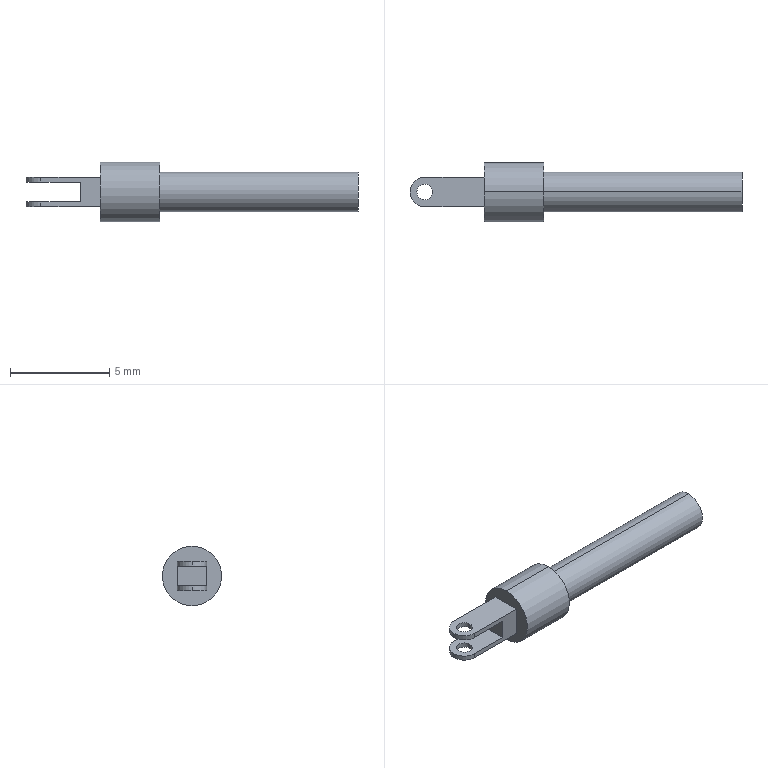Part | SolidWorks | features ICE 3, Revolution 1 | 1 solid | 25 faces | box 16.75 x 3 x 3 mm | volume 51.85 mm3 | cylinder 14 | plane 11 | commonest cylinder face diameters 0.8 x4 1.5 x4 1 x2 2 x2 3 x2
STEP:
#1=CARTESIAN_POINT('',(7.,0.,0.5));
#2=VERTEX_POINT('',#1);
#3=CARTESIAN_POINT('',(7.,0.,-0.5));
#4=VERTEX_POINT('',#3);
#5=CARTESIAN_POINT('',(7.,0.,0.));
#6=DIRECTION('',(1.,0.,0.));
#7=DIRECTION('',(0.,0.,-1.));
#8=AXIS2_PLACEMENT_3D('',#5,#6,#7);
#9=CIRCLE('',#8,0.5);
#10=EDGE_CURVE('',#2,#4,#9,.T.);
#11=ORIENTED_EDGE('',*,*,#10,.F.);
#12=CARTESIAN_POINT('',(13.,0.,0.5));
#13=VERTEX_POINT('',#12);
#14=CARTESIAN_POINT('',(7.,0.,0.5));
#15=DIRECTION('',(1.,0.,0.));
#16=VECTOR('',#15,1000.);
#17=LINE('',#14,#16);
#18=EDGE_CURVE('',#2,#13,#17,.T.);
#19=ORIENTED_EDGE('',*,*,#18,.T.);
#20=CARTESIAN_POINT('',(13.,0.,-0.5));
#21=VERTEX_POINT('',#20);
#22=CARTESIAN_POINT('',(13.,0.,0.));
#23=DIRECTION('',(1.,0.,0.));
#24=DIRECTION('',(0.,0.,-1.));
#25=AXIS2_PLACEMENT_3D('',#22,#23,#24);
#26=CIRCLE('',#25,0.5);
#27=EDGE_CURVE('',#13,#21,#26,.T.);
#28=ORIENTED_EDGE('',*,*,#27,.T.);
#29=CARTESIAN_POINT('',(7.,0.,-0.5));
#30=DIRECTION('',(1.,0.,0.));
#31=VECTOR('',#30,1000.);
#32=LINE('',#29,#31);
#33=EDGE_CURVE('',#4,#21,#32,.T.);
#34=ORIENTED_EDGE('',*,*,#33,.F.);
#35=EDGE_LOOP('',(#11,#19,#28,#34));
#36=FACE_OUTER_BOUND('',#35,.T.);
#37=CARTESIAN_POINT('',(7.,0.,0.));
#38=DIRECTION('',(1.,0.,0.));
#39=DIRECTION('',(0.,0.,-1.));
#40=AXIS2_PLACEMENT_3D('',#37,#38,#39);
#41=CYLINDRICAL_SURFACE('',#40,0.5);
#42=ADVANCED_FACE('',(#36),#41,.F.);
#43=CARTESIAN_POINT('',(-2.6,0.,-0.5));
#44=VERTEX_POINT('',#43);
#45=CARTESIAN_POINT('',(-3.4,0.,-0.5));
#46=VERTEX_POINT('',#45);
#47=CARTESIAN_POINT('',(-3.,0.,-0.5));
#48=DIRECTION('',(0.,0.,-1.));
#49=DIRECTION('',(-1.,0.,0.));
#50=AXIS2_PLACEMENT_3D('',#47,#48,#49);
#51=CIRCLE('',#50,0.4);
#52=EDGE_CURVE('',#44,#46,#51,.T.);
#53=ORIENTED_EDGE('',*,*,#52,.F.);
#54=CARTESIAN_POINT('',(-2.6,0.,-0.75));
#55=VERTEX_POINT('',#54);
#56=CARTESIAN_POINT('',(-2.6,0.,0.75));
#57=DIRECTION('',(0.,0.,-1.));
#58=VECTOR('',#57,1000.);
#59=LINE('',#56,#58);
#60=EDGE_CURVE('',#44,#55,#59,.T.);
#61=ORIENTED_EDGE('',*,*,#60,.T.);
#62=CARTESIAN_POINT('',(-3.4,0.,-0.75));
#63=VERTEX_POINT('',#62);
#64=CARTESIAN_POINT('',(-3.,0.,-0.75));
#65=DIRECTION('',(0.,0.,1.));
#66=DIRECTION('',(1.,0.,0.));
#67=AXIS2_PLACEMENT_3D('',#64,#65,#66);
#68=CIRCLE('',#67,0.4);
#69=EDGE_CURVE('',#63,#55,#68,.T.);
#70=ORIENTED_EDGE('',*,*,#69,.F.);
#71=CARTESIAN_POINT('',(-3.4,0.,0.75));
#72=DIRECTION('',(0.,0.,-1.));
#73=VECTOR('',#72,1000.);
#74=LINE('',#71,#73);
#75=EDGE_CURVE('',#46,#63,#74,.T.);
#76=ORIENTED_EDGE('',*,*,#75,.F.);
#77=EDGE_LOOP('',(#53,#61,#70,#76));
#78=FACE_OUTER_BOUND('',#77,.T.);
#79=CARTESIAN_POINT('',(-3.,0.,0.75));
#80=DIRECTION('',(0.,0.,-1.));
#81=DIRECTION('',(-1.,0.,0.));
#82=AXIS2_PLACEMENT_3D('',#79,#80,#81);
#83=CYLINDRICAL_SURFACE('',#82,0.4);
#84=ADVANCED_FACE('',(#78),#83,.F.);
#85=CARTESIAN_POINT('',(-3.75,0.,-0.5));
#86=VERTEX_POINT('',#85);
#87=CARTESIAN_POINT('',(-3.,-0.75,-0.5));
#88=VERTEX_POINT('',#87);
#89=CARTESIAN_POINT('',(-3.,0.,-0.5));
#90=DIRECTION('',(0.,0.,1.));
#91=DIRECTION('',(-1.,0.,0.));
#92=AXIS2_PLACEMENT_3D('',#89,#90,#91);
#93=CIRCLE('',#92,0.75);
#94=EDGE_CURVE('',#86,#88,#93,.T.);
#95=ORIENTED_EDGE('',*,*,#94,.F.);
#96=CARTESIAN_POINT('',(-3.75,0.,-0.75));
#97=VERTEX_POINT('',#96);
#98=CARTESIAN_POINT('',(-3.75,0.,0.75));
#99=DIRECTION('',(0.,0.,-1.));
#100=VECTOR('',#99,1000.);
#101=LINE('',#98,#100);
#102=EDGE_CURVE('',#86,#97,#101,.T.);
#103=ORIENTED_EDGE('',*,*,#102,.T.);
#104=CARTESIAN_POINT('',(-3.,-0.75,-0.75));
#105=VERTEX_POINT('',#104);
#106=CARTESIAN_POINT('',(-3.,0.,-0.75));
#107=DIRECTION('',(0.,0.,1.));
#108=DIRECTION('',(-1.,0.,0.));
#109=AXIS2_PLACEMENT_3D('',#106,#107,#108);
#110=CIRCLE('',#109,0.75);
#111=EDGE_CURVE('',#97,#105,#110,.T.);
#112=ORIENTED_EDGE('',*,*,#111,.T.);
#113=CARTESIAN_POINT('',(-3.,-0.75,0.75));
#114=DIRECTION('',(0.,0.,-1.));
#115=VECTOR('',#114,1000.);
#116=LINE('',#113,#115);
#117=EDGE_CURVE('',#88,#105,#116,.T.);
#118=ORIENTED_EDGE('',*,*,#117,.F.);
#119=EDGE_LOOP('',(#95,#103,#112,#118));
#120=FACE_OUTER_BOUND('',#119,.T.);
#121=CARTESIAN_POINT('',(-3.,0.,0.75));
#122=DIRECTION('',(0.,0.,-1.));
#123=DIRECTION('',(-1.,0.,0.));
#124=AXIS2_PLACEMENT_3D('',#121,#122,#123);
#125=CYLINDRICAL_SURFACE('',#124,0.75);
#126=ADVANCED_FACE('',(#120),#125,.T.);
#127=CARTESIAN_POINT('',(13.,0.,1.));
#128=VERTEX_POINT('',#127);
#129=CARTESIAN_POINT('',(13.,0.,-1.));
#130=VERTEX_POINT('',#129);
#131=CARTESIAN_POINT('',(13.,0.,0.));
#132=DIRECTION('',(-1.,0.,0.));
#133=DIRECTION('',(0.,0.,1.));
#134=AXIS2_PLACEMENT_3D('',#131,#132,#133);
#135=CIRCLE('',#134,1.);
#136=EDGE_CURVE('',#128,#130,#135,.T.);
#137=ORIENTED_EDGE('',*,*,#136,.T.);
#138=CARTESIAN_POINT('',(3.,0.,-1.));
#139=VERTEX_POINT('',#138);
#140=CARTESIAN_POINT('',(0.1244,0.,-1.));
#141=DIRECTION('',(-1.,0.,0.));
#142=VECTOR('',#141,1000.);
#143=LINE('',#140,#142);
#144=EDGE_CURVE('',#130,#139,#143,.T.);
#145=ORIENTED_EDGE('',*,*,#144,.T.);
#146=CARTESIAN_POINT('',(3.,0.,1.));
#147=VERTEX_POINT('',#146);
#148=CARTESIAN_POINT('',(3.,0.,0.));
#149=DIRECTION('',(-1.,0.,0.));
#150=DIRECTION('',(0.,0.,1.));
#151=AXIS2_PLACEMENT_3D('',#148,#149,#150);
#152=CIRCLE('',#151,1.);
#153=EDGE_CURVE('',#147,#139,#152,.T.);
#154=ORIENTED_EDGE('',*,*,#153,.F.);
#155=CARTESIAN_POINT('',(0.1244,0.,1.));
#156=DIRECTION('',(-1.,0.,0.));
#157=VECTOR('',#156,1000.);
#158=LINE('',#155,#157);
#159=EDGE_CURVE('',#128,#147,#158,.T.);
#160=ORIENTED_EDGE('',*,*,#159,.F.);
#161=EDGE_LOOP('',(#137,#145,#154,#160));
#162=FACE_OUTER_BOUND('',#161,.T.);
#163=CARTESIAN_POINT('',(0.1244,0.,0.));
#164=DIRECTION('',(-1.,0.,0.));
#165=DIRECTION('',(0.,0.,1.));
#166=AXIS2_PLACEMENT_3D('',#163,#164,#165);
#167=CYLINDRICAL_SURFACE('',#166,1.);
#168=ADVANCED_FACE('',(#162),#167,.T.);
#169=CARTESIAN_POINT('',(3.,0.,1.5));
#170=VERTEX_POINT('',#169);
#171=CARTESIAN_POINT('',(3.,0.,-1.5));
#172=VERTEX_POINT('',#171);
#173=CARTESIAN_POINT('',(3.,0.,0.));
#174=DIRECTION('',(-1.,0.,0.));
#175=DIRECTION('',(0.,0.,1.));
#176=AXIS2_PLACEMENT_3D('',#173,#174,#175);
#177=CIRCLE('',#176,1.5);
#178=EDGE_CURVE('',#170,#172,#177,.T.);
#179=ORIENTED_EDGE('',*,*,#178,.T.);
#180=CARTESIAN_POINT('',(0.,0.,-1.5));
#181=VERTEX_POINT('',#180);
#182=CARTESIAN_POINT('',(0.1244,0.,-1.5));
#183=DIRECTION('',(-1.,0.,0.));
#184=VECTOR('',#183,1000.);
#185=LINE('',#182,#184);
#186=EDGE_CURVE('',#172,#181,#185,.T.);
#187=ORIENTED_EDGE('',*,*,#186,.T.);
#188=CARTESIAN_POINT('',(0.,0.,1.5));
#189=VERTEX_POINT('',#188);
#190=CARTESIAN_POINT('',(0.,0.,0.));
#191=DIRECTION('',(-1.,0.,0.));
#192=DIRECTION('',(0.,0.,1.));
#193=AXIS2_PLACEMENT_3D('',#190,#191,#192);
#194=CIRCLE('',#193,1.5);
#195=EDGE_CURVE('',#189,#181,#194,.T.);
#196=ORIENTED_EDGE('',*,*,#195,.F.);
#197=CARTESIAN_POINT('',(0.1244,0.,1.5));
#198=DIRECTION('',(-1.,0.,0.));
#199=VECTOR('',#198,1000.);
#200=LINE('',#197,#199);
#201=EDGE_CURVE('',#170,#189,#200,.T.);
#202=ORIENTED_EDGE('',*,*,#201,.F.);
#203=EDGE_LOOP('',(#179,#187,#196,#202));
#204=FACE_OUTER_BOUND('',#203,.T.);
#205=CARTESIAN_POINT('',(0.1244,0.,0.));
#206=DIRECTION('',(-1.,0.,0.));
#207=DIRECTION('',(0.,0.,1.));
#208=AXIS2_PLACEMENT_3D('',#205,#206,#207);
#209=CYLINDRICAL_SURFACE('',#208,1.5);
#210=ADVANCED_FACE('',(#204),#209,.T.);
#211=CARTESIAN_POINT('',(-3.4,0.,0.75));
#212=VERTEX_POINT('',#211);
#213=CARTESIAN_POINT('',(-2.6,0.,0.75));
#214=VERTEX_POINT('',#213);
#215=CARTESIAN_POINT('',(-3.,0.,0.75));
#216=DIRECTION('',(0.,0.,1.));
#217=DIRECTION('',(1.,0.,0.));
#218=AXIS2_PLACEMENT_3D('',#215,#216,#217);
#219=CIRCLE('',#218,0.4);
#220=EDGE_CURVE('',#212,#214,#219,.T.);
#221=ORIENTED_EDGE('',*,*,#220,.T.);
#222=CARTESIAN_POINT('',(-2.6,0.,0.5));
#223=VERTEX_POINT('',#222);
#224=CARTESIAN_POINT('',(-2.6,0.,0.75));
#225=DIRECTION('',(0.,0.,-1.));
#226=VECTOR('',#225,1000.);
#227=LINE('',#224,#226);
#228=EDGE_CURVE('',#214,#223,#227,.T.);
#229=ORIENTED_EDGE('',*,*,#228,.T.);
#230=CARTESIAN_POINT('',(-3.4,0.,0.5));
#231=VERTEX_POINT('',#230);
#232=CARTESIAN_POINT('',(-3.,0.,0.5));
#233=DIRECTION('',(0.,0.,-1.));
#234=DIRECTION('',(-1.,0.,0.));
#235=AXIS2_PLACEMENT_3D('',#232,#233,#234);
#236=CIRCLE('',#235,0.4);
#237=EDGE_CURVE('',#223,#231,#236,.T.);
#238=ORIENTED_EDGE('',*,*,#237,.T.);
#239=CARTESIAN_POINT('',(-3.4,0.,0.75));
#240=DIRECTION('',(0.,0.,-1.));
#241=VECTOR('',#240,1000.);
#242=LINE('',#239,#241);
#243=EDGE_CURVE('',#212,#231,#242,.T.);
#244=ORIENTED_EDGE('',*,*,#243,.F.);
#245=EDGE_LOOP('',(#221,#229,#238,#244));
#246=FACE_OUTER_BOUND('',#245,.T.);
#247=CARTESIAN_POINT('',(-3.,0.,0.75));
#248=DIRECTION('',(0.,0.,-1.));
#249=DIRECTION('',(-1.,0.,0.));
#250=AXIS2_PLACEMENT_3D('',#247,#248,#249);
#251=CYLINDRICAL_SURFACE('',#250,0.4);
#252=ADVANCED_FACE('',(#246),#251,.F.);
#253=CARTESIAN_POINT('',(-3.75,0.,0.75));
#254=VERTEX_POINT('',#253);
#255=CARTESIAN_POINT('',(-3.,-0.75,0.75));
#256=VERTEX_POINT('',#255);
#257=CARTESIAN_POINT('',(-3.,0.,0.75));
#258=DIRECTION('',(0.,0.,1.));
#259=DIRECTION('',(-1.,0.,0.));
#260=AXIS2_PLACEMENT_3D('',#257,#258,#259);
#261=CIRCLE('',#260,0.75);
#262=EDGE_CURVE('',#254,#256,#261,.T.);
#263=ORIENTED_EDGE('',*,*,#262,.F.);
#264=CARTESIAN_POINT('',(-3.75,0.,0.5));
#265=VERTEX_POINT('',#264);
#266=CARTESIAN_POINT('',(-3.75,0.,0.75));
#267=DIRECTION('',(0.,0.,-1.));
#268=VECTOR('',#267,1000.);
#269=LINE('',#266,#268);
#270=EDGE_CURVE('',#254,#265,#269,.T.);
#271=ORIENTED_EDGE('',*,*,#270,.T.);
#272=CARTESIAN_POINT('',(-3.,-0.75,0.5));
#273=VERTEX_POINT('',#272);
#274=CARTESIAN_POINT('',(-3.,0.,0.5));
#275=DIRECTION('',(0.,0.,1.));
#276=DIRECTION('',(-1.,0.,0.));
#277=AXIS2_PLACEMENT_3D('',#274,#275,#276);
#278=CIRCLE('',#277,0.75);
#279=EDGE_CURVE('',#265,#273,#278,.T.);
#280=ORIENTED_EDGE('',*,*,#279,.T.);
#281=CARTESIAN_POINT('',(-3.,-0.75,0.75));
#282=DIRECTION('',(0.,0.,-1.));
#283=VECTOR('',#282,1000.);
#284=LINE('',#281,#283);
#285=EDGE_CURVE('',#256,#273,#284,.T.);
#286=ORIENTED_EDGE('',*,*,#285,.F.);
#287=EDGE_LOOP('',(#263,#271,#280,#286));
#288=FACE_OUTER_BOUND('',#287,.T.);
#289=CARTESIAN_POINT('',(-3.,0.,0.75));
#290=DIRECTION('',(0.,0.,-1.));
#291=DIRECTION('',(-1.,0.,0.));
#292=AXIS2_PLACEMENT_3D('',#289,#290,#291);
#293=CYLINDRICAL_SURFACE('',#292,0.75);
#294=ADVANCED_FACE('',(#288),#293,.T.);
#295=ORIENTED_EDGE('',*,*,#270,.F.);
#296=CARTESIAN_POINT('',(-3.,0.75,0.75));
#297=VERTEX_POINT('',#296);
#298=CARTESIAN_POINT('',(-3.,0.,0.75));
#299=DIRECTION('',(0.,0.,1.));
#300=DIRECTION('',(-1.,0.,0.));
#301=AXIS2_PLACEMENT_3D('',#298,#299,#300);
#302=CIRCLE('',#301,0.75);
#303=EDGE_CURVE('',#297,#254,#302,.T.);
#304=ORIENTED_EDGE('',*,*,#303,.F.);
#305=CARTESIAN_POINT('',(-3.,0.75,0.5));
#306=VERTEX_POINT('',#305);
#307=CARTESIAN_POINT('',(-3.,0.75,0.75));
#308=DIRECTION('',(0.,0.,-1.));
#309=VECTOR('',#308,1000.);
#310=LINE('',#307,#309);
#311=EDGE_CURVE('',#297,#306,#310,.T.);
#312=ORIENTED_EDGE('',*,*,#311,.T.);
#313=CARTESIAN_POINT('',(-3.,0.,0.5));
#314=DIRECTION('',(0.,0.,1.));
#315=DIRECTION('',(-1.,0.,0.));
#316=AXIS2_PLACEMENT_3D('',#313,#314,#315);
#317=CIRCLE('',#316,0.75);
#318=EDGE_CURVE('',#306,#265,#317,.T.);
#319=ORIENTED_EDGE('',*,*,#318,.T.);
#320=EDGE_LOOP('',(#295,#304,#312,#319));
#321=FACE_OUTER_BOUND('',#320,.T.);
#322=CARTESIAN_POINT('',(-3.,0.,0.75));
#323=DIRECTION('',(0.,0.,-1.));
#324=DIRECTION('',(-1.,0.,0.));
#325=AXIS2_PLACEMENT_3D('',#322,#323,#324);
#326=CYLINDRICAL_SURFACE('',#325,0.75);
#327=ADVANCED_FACE('',(#321),#326,.T.);
#328=ORIENTED_EDGE('',*,*,#228,.F.);
#329=CARTESIAN_POINT('',(-3.,0.,0.75));
#330=DIRECTION('',(0.,0.,1.));
#331=DIRECTION('',(1.,0.,0.));
#332=AXIS2_PLACEMENT_3D('',#329,#330,#331);
#333=CIRCLE('',#332,0.4);
#334=EDGE_CURVE('',#214,#212,#333,.T.);
#335=ORIENTED_EDGE('',*,*,#334,.T.);
#336=ORIENTED_EDGE('',*,*,#243,.T.);
#337=CARTESIAN_POINT('',(-3.,0.,0.5));
#338=DIRECTION('',(0.,0.,-1.));
#339=DIRECTION('',(-1.,0.,0.));
#340=AXIS2_PLACEMENT_3D('',#337,#338,#339);
#341=CIRCLE('',#340,0.4);
#342=EDGE_CURVE('',#231,#223,#341,.T.);
#343=ORIENTED_EDGE('',*,*,#342,.T.);
#344=EDGE_LOOP('',(#328,#335,#336,#343));
#345=FACE_OUTER_BOUND('',#344,.T.);
#346=CARTESIAN_POINT('',(-3.,0.,0.75));
#347=DIRECTION('',(0.,0.,-1.));
#348=DIRECTION('',(-1.,0.,0.));
#349=AXIS2_PLACEMENT_3D('',#346,#347,#348);
#350=CYLINDRICAL_SURFACE('',#349,0.4);
#351=ADVANCED_FACE('',(#345),#350,.F.);
#352=CARTESIAN_POINT('',(0.,-0.75,0.75));
#353=VERTEX_POINT('',#352);
#354=CARTESIAN_POINT('',(0.,-0.75,-0.75));
#355=VERTEX_POINT('',#354);
#356=CARTESIAN_POINT('',(0.,-0.75,0.75));
#357=DIRECTION('',(0.,0.,-1.));
#358=VECTOR('',#357,1000.);
#359=LINE('',#356,#358);
#360=EDGE_CURVE('',#353,#355,#359,.T.);
#361=ORIENTED_EDGE('',*,*,#360,.T.);
#362=CARTESIAN_POINT('',(0.,0.75,-0.75));
#363=VERTEX_POINT('',#362);
#364=CARTESIAN_POINT('',(0.,0.75,-0.75));
#365=DIRECTION('',(0.,1.,0.));
#366=VECTOR('',#365,1000.);
#367=LINE('',#364,#366);
#368=EDGE_CURVE('',#355,#363,#367,.T.);
#369=ORIENTED_EDGE('',*,*,#368,.T.);
#370=CARTESIAN_POINT('',(0.,0.75,0.75));
#371=VERTEX_POINT('',#370);
#372=CARTESIAN_POINT('',(0.,0.75,0.75));
#373=DIRECTION('',(0.,0.,-1.));
#374=VECTOR('',#373,1000.);
#375=LINE('',#372,#374);
#376=EDGE_CURVE('',#371,#363,#375,.T.);
#377=ORIENTED_EDGE('',*,*,#376,.F.);
#378=CARTESIAN_POINT('',(0.,0.75,0.75));
#379=DIRECTION('',(0.,1.,0.));
#380=VECTOR('',#379,1000.);
#381=LINE('',#378,#380);
#382=EDGE_CURVE('',#353,#371,#381,.T.);
#383=ORIENTED_EDGE('',*,*,#382,.F.);
#384=EDGE_LOOP('',(#361,#369,#377,#383));
#385=FACE_BOUND('',#384,.T.);
#386=ORIENTED_EDGE('',*,*,#195,.T.);
#387=CARTESIAN_POINT('',(0.,0.,0.));
#388=DIRECTION('',(-1.,0.,0.));
#389=DIRECTION('',(0.,0.,1.));
#390=AXIS2_PLACEMENT_3D('',#387,#388,#389);
#391=CIRCLE('',#390,1.5);
#392=EDGE_CURVE('',#181,#189,#391,.T.);
#393=ORIENTED_EDGE('',*,*,#392,.T.);
#394=EDGE_LOOP('',(#386,#393));
#395=FACE_OUTER_BOUND('',#394,.T.);
#396=CARTESIAN_POINT('',(0.,0.,0.));
#397=DIRECTION('',(1.,0.,0.));
#398=DIRECTION('',(0.,0.,-1.));
#399=AXIS2_PLACEMENT_3D('',#396,#397,#398);
#400=PLANE('',#399);
#401=ADVANCED_FACE('',(#385,#395),#400,.F.);
#402=ORIENTED_EDGE('',*,*,#186,.F.);
#403=CARTESIAN_POINT('',(3.,0.,0.));
#404=DIRECTION('',(-1.,0.,0.));
#405=DIRECTION('',(0.,0.,1.));
#406=AXIS2_PLACEMENT_3D('',#403,#404,#405);
#407=CIRCLE('',#406,1.5);
#408=EDGE_CURVE('',#172,#170,#407,.T.);
#409=ORIENTED_EDGE('',*,*,#408,.T.);
#410=ORIENTED_EDGE('',*,*,#201,.T.);
#411=ORIENTED_EDGE('',*,*,#392,.F.);
#412=EDGE_LOOP('',(#402,#409,#410,#411));
#413=FACE_OUTER_BOUND('',#412,.T.);
#414=CARTESIAN_POINT('',(0.1244,0.,0.));
#415=DIRECTION('',(-1.,0.,0.));
#416=DIRECTION('',(0.,0.,1.));
#417=AXIS2_PLACEMENT_3D('',#414,#415,#416);
#418=CYLINDRICAL_SURFACE('',#417,1.5);
#419=ADVANCED_FACE('',(#413),#418,.T.);
#420=ORIENTED_EDGE('',*,*,#178,.F.);
#421=ORIENTED_EDGE('',*,*,#408,.F.);
#422=EDGE_LOOP('',(#420,#421));
#423=FACE_OUTER_BOUND('',#422,.T.);
#424=ORIENTED_EDGE('',*,*,#153,.T.);
#425=CARTESIAN_POINT('',(3.,0.,0.));
#426=DIRECTION('',(-1.,0.,0.));
#427=DIRECTION('',(0.,0.,1.));
#428=AXIS2_PLACEMENT_3D('',#425,#426,#427);
#429=CIRCLE('',#428,1.);
#430=EDGE_CURVE('',#139,#147,#429,.T.);
#431=ORIENTED_EDGE('',*,*,#430,.T.);
#432=EDGE_LOOP('',(#424,#431));
#433=FACE_BOUND('',#432,.T.);
#434=CARTESIAN_POINT('',(3.,1.5,0.));
#435=DIRECTION('',(-1.,0.,0.));
#436=DIRECTION('',(0.,0.,1.));
#437=AXIS2_PLACEMENT_3D('',#434,#435,#436);
#438=PLANE('',#437);
#439=ADVANCED_FACE('',(#423,#433),#438,.F.);
#440=ORIENTED_EDGE('',*,*,#144,.F.);
#441=CARTESIAN_POINT('',(13.,0.,0.));
#442=DIRECTION('',(-1.,0.,0.));
#443=DIRECTION('',(0.,0.,1.));
#444=AXIS2_PLACEMENT_3D('',#441,#442,#443);
#445=CIRCLE('',#444,1.);
#446=EDGE_CURVE('',#130,#128,#445,.T.);
#447=ORIENTED_EDGE('',*,*,#446,.T.);
#448=ORIENTED_EDGE('',*,*,#159,.T.);
#449=ORIENTED_EDGE('',*,*,#430,.F.);
#450=EDGE_LOOP('',(#440,#447,#448,#449));
#451=FACE_OUTER_BOUND('',#450,.T.);
#452=CARTESIAN_POINT('',(0.1244,0.,0.));
#453=DIRECTION('',(-1.,0.,0.));
#454=DIRECTION('',(0.,0.,1.));
#455=AXIS2_PLACEMENT_3D('',#452,#453,#454);
#456=CYLINDRICAL_SURFACE('',#455,1.);
#457=ADVANCED_FACE('',(#451),#456,.T.);
#458=CARTESIAN_POINT('',(13.,0.,0.));
#459=DIRECTION('',(1.,0.,0.));
#460=DIRECTION('',(0.,0.,-1.));
#461=AXIS2_PLACEMENT_3D('',#458,#459,#460);
#462=CIRCLE('',#461,0.5);
#463=EDGE_CURVE('',#21,#13,#462,.T.);
#464=ORIENTED_EDGE('',*,*,#463,.F.);
#465=ORIENTED_EDGE('',*,*,#27,.F.);
#466=EDGE_LOOP('',(#464,#465));
#467=FACE_BOUND('',#466,.T.);
#468=ORIENTED_EDGE('',*,*,#136,.F.);
#469=ORIENTED_EDGE('',*,*,#446,.F.);
#470=EDGE_LOOP('',(#468,#469));
#471=FACE_OUTER_BOUND('',#470,.T.);
#472=CARTESIAN_POINT('',(13.,1.,0.));
#473=DIRECTION('',(-1.,0.,0.));
#474=DIRECTION('',(0.,0.,1.));
#475=AXIS2_PLACEMENT_3D('',#472,#473,#474);
#476=PLANE('',#475);
#477=ADVANCED_FACE('',(#467,#471),#476,.F.);
#478=CARTESIAN_POINT('',(0.,-0.75,0.75));
#479=DIRECTION('',(1.,0.,0.));
#480=VECTOR('',#479,1000.);
#481=LINE('',#478,#480);
#482=EDGE_CURVE('',#256,#353,#481,.T.);
#483=ORIENTED_EDGE('',*,*,#482,.T.);
#484=ORIENTED_EDGE('',*,*,#382,.T.);
#485=CARTESIAN_POINT('',(0.,0.75,0.75));
#486=DIRECTION('',(-1.,0.,0.));
#487=VECTOR('',#486,1000.);
#488=LINE('',#485,#487);
#489=EDGE_CURVE('',#371,#297,#488,.T.);
#490=ORIENTED_EDGE('',*,*,#489,.T.);
#491=ORIENTED_EDGE('',*,*,#303,.T.);
#492=ORIENTED_EDGE('',*,*,#262,.T.);
#493=EDGE_LOOP('',(#483,#484,#490,#491,#492));
#494=FACE_OUTER_BOUND('',#493,.T.);
#495=ORIENTED_EDGE('',*,*,#220,.F.);
#496=ORIENTED_EDGE('',*,*,#334,.F.);
#497=EDGE_LOOP('',(#495,#496));
#498=FACE_BOUND('',#497,.T.);
#499=CARTESIAN_POINT('',(-3.,0.,0.75));
#500=DIRECTION('',(0.,0.,-1.));
#501=DIRECTION('',(-1.,0.,0.));
#502=AXIS2_PLACEMENT_3D('',#499,#500,#501);
#503=PLANE('',#502);
#504=ADVANCED_FACE('',(#494,#498),#503,.F.);
#505=CARTESIAN_POINT('',(0.,-0.75,-0.75));
#506=DIRECTION('',(1.,0.,0.));
#507=VECTOR('',#506,1000.);
#508=LINE('',#505,#507);
#509=EDGE_CURVE('',#105,#355,#508,.T.);
#510=ORIENTED_EDGE('',*,*,#509,.F.);
#511=ORIENTED_EDGE('',*,*,#111,.F.);
#512=CARTESIAN_POINT('',(-3.,0.75,-0.75));
#513=VERTEX_POINT('',#512);
#514=CARTESIAN_POINT('',(-3.,0.,-0.75));
#515=DIRECTION('',(0.,0.,1.));
#516=DIRECTION('',(-1.,0.,0.));
#517=AXIS2_PLACEMENT_3D('',#514,#515,#516);
#518=CIRCLE('',#517,0.75);
#519=EDGE_CURVE('',#513,#97,#518,.T.);
#520=ORIENTED_EDGE('',*,*,#519,.F.);
#521=CARTESIAN_POINT('',(0.,0.75,-0.75));
#522=DIRECTION('',(-1.,0.,0.));
#523=VECTOR('',#522,1000.);
#524=LINE('',#521,#523);
#525=EDGE_CURVE('',#363,#513,#524,.T.);
#526=ORIENTED_EDGE('',*,*,#525,.F.);
#527=ORIENTED_EDGE('',*,*,#368,.F.);
#528=EDGE_LOOP('',(#510,#511,#520,#526,#527));
#529=FACE_OUTER_BOUND('',#528,.T.);
#530=ORIENTED_EDGE('',*,*,#69,.T.);
#531=CARTESIAN_POINT('',(-3.,0.,-0.75));
#532=DIRECTION('',(0.,0.,1.));
#533=DIRECTION('',(1.,0.,0.));
#534=AXIS2_PLACEMENT_3D('',#531,#532,#533);
#535=CIRCLE('',#534,0.4);
#536=EDGE_CURVE('',#55,#63,#535,.T.);
#537=ORIENTED_EDGE('',*,*,#536,.T.);
#538=EDGE_LOOP('',(#530,#537));
#539=FACE_BOUND('',#538,.T.);
#540=CARTESIAN_POINT('',(-3.,0.,-0.75));
#541=DIRECTION('',(0.,0.,-1.));
#542=DIRECTION('',(-1.,0.,0.));
#543=AXIS2_PLACEMENT_3D('',#540,#541,#542);
#544=PLANE('',#543);
#545=ADVANCED_FACE('',(#529,#539),#544,.T.);
#546=CARTESIAN_POINT('',(-1.,-0.75,-0.5));
#547=VERTEX_POINT('',#546);
#548=CARTESIAN_POINT('',(-1.,-0.75,0.5));
#549=VERTEX_POINT('',#548);
#550=CARTESIAN_POINT('',(-1.,-0.75,-0.5));
#551=DIRECTION('',(0.,0.,1.));
#552=VECTOR('',#551,1000.);
#553=LINE('',#550,#552);
#554=EDGE_CURVE('',#547,#549,#553,.T.);
#555=ORIENTED_EDGE('',*,*,#554,.F.);
#556=CARTESIAN_POINT('',(-1.,-0.75,-0.5));
#557=DIRECTION('',(1.,0.,0.));
#558=VECTOR('',#557,1000.);
#559=LINE('',#556,#558);
#560=EDGE_CURVE('',#88,#547,#559,.T.);
#561=ORIENTED_EDGE('',*,*,#560,.F.);
#562=ORIENTED_EDGE('',*,*,#117,.T.);
#563=ORIENTED_EDGE('',*,*,#509,.T.);
#564=ORIENTED_EDGE('',*,*,#360,.F.);
#565=ORIENTED_EDGE('',*,*,#482,.F.);
#566=ORIENTED_EDGE('',*,*,#285,.T.);
#567=CARTESIAN_POINT('',(-1.,-0.75,0.5));
#568=DIRECTION('',(1.,0.,0.));
#569=VECTOR('',#568,1000.);
#570=LINE('',#567,#569);
#571=EDGE_CURVE('',#273,#549,#570,.T.);
#572=ORIENTED_EDGE('',*,*,#571,.T.);
#573=EDGE_LOOP('',(#555,#561,#562,#563,#564,#565,#566,#572));
#574=FACE_OUTER_BOUND('',#573,.T.);
#575=CARTESIAN_POINT('',(0.,-0.75,0.75));
#576=DIRECTION('',(0.,1.,0.));
#577=DIRECTION('',(-1.,0.,0.));
#578=AXIS2_PLACEMENT_3D('',#575,#576,#577);
#579=PLANE('',#578);
#580=ADVANCED_FACE('',(#574),#579,.F.);
#581=CARTESIAN_POINT('',(-3.,0.75,-0.5));
#582=VERTEX_POINT('',#581);
#583=CARTESIAN_POINT('',(-3.,0.75,0.75));
#584=DIRECTION('',(0.,0.,-1.));
#585=VECTOR('',#584,1000.);
#586=LINE('',#583,#585);
#587=EDGE_CURVE('',#582,#513,#586,.T.);
#588=ORIENTED_EDGE('',*,*,#587,.F.);
#589=CARTESIAN_POINT('',(-1.,0.75,-0.5));
#590=VERTEX_POINT('',#589);
#591=CARTESIAN_POINT('',(-3.,0.75,-0.5));
#592=DIRECTION('',(-1.,0.,0.));
#593=VECTOR('',#592,1000.);
#594=LINE('',#591,#593);
#595=EDGE_CURVE('',#590,#582,#594,.T.);
#596=ORIENTED_EDGE('',*,*,#595,.F.);
#597=CARTESIAN_POINT('',(-1.,0.75,0.5));
#598=VERTEX_POINT('',#597);
#599=CARTESIAN_POINT('',(-1.,0.75,-0.5));
#600=DIRECTION('',(0.,0.,1.));
#601=VECTOR('',#600,1000.);
#602=LINE('',#599,#601);
#603=EDGE_CURVE('',#590,#598,#602,.T.);
#604=ORIENTED_EDGE('',*,*,#603,.T.);
#605=CARTESIAN_POINT('',(-3.,0.75,0.5));
#606=DIRECTION('',(-1.,0.,0.));
#607=VECTOR('',#606,1000.);
#608=LINE('',#605,#607);
#609=EDGE_CURVE('',#598,#306,#608,.T.);
#610=ORIENTED_EDGE('',*,*,#609,.T.);
#611=ORIENTED_EDGE('',*,*,#311,.F.);
#612=ORIENTED_EDGE('',*,*,#489,.F.);
#613=ORIENTED_EDGE('',*,*,#376,.T.);
#614=ORIENTED_EDGE('',*,*,#525,.T.);
#615=EDGE_LOOP('',(#588,#596,#604,#610,#611,#612,#613,#614));
#616=FACE_OUTER_BOUND('',#615,.T.);
#617=CARTESIAN_POINT('',(0.,0.75,0.75));
#618=DIRECTION('',(0.,-1.,0.));
#619=DIRECTION('',(1.,0.,0.));
#620=AXIS2_PLACEMENT_3D('',#617,#618,#619);
#621=PLANE('',#620);
#622=ADVANCED_FACE('',(#616),#621,.F.);
#623=ORIENTED_EDGE('',*,*,#102,.F.);
#624=CARTESIAN_POINT('',(-3.,0.,-0.5));
#625=DIRECTION('',(0.,0.,1.));
#626=DIRECTION('',(-1.,0.,0.));
#627=AXIS2_PLACEMENT_3D('',#624,#625,#626);
#628=CIRCLE('',#627,0.75);
#629=EDGE_CURVE('',#582,#86,#628,.T.);
#630=ORIENTED_EDGE('',*,*,#629,.F.);
#631=ORIENTED_EDGE('',*,*,#587,.T.);
#632=ORIENTED_EDGE('',*,*,#519,.T.);
#633=EDGE_LOOP('',(#623,#630,#631,#632));
#634=FACE_OUTER_BOUND('',#633,.T.);
#635=CARTESIAN_POINT('',(-3.,0.,0.75));
#636=DIRECTION('',(0.,0.,-1.));
#637=DIRECTION('',(-1.,0.,0.));
#638=AXIS2_PLACEMENT_3D('',#635,#636,#637);
#639=CYLINDRICAL_SURFACE('',#638,0.75);
#640=ADVANCED_FACE('',(#634),#639,.T.);
#641=ORIENTED_EDGE('',*,*,#60,.F.);
#642=CARTESIAN_POINT('',(-3.,0.,-0.5));
#643=DIRECTION('',(0.,0.,-1.));
#644=DIRECTION('',(-1.,0.,0.));
#645=AXIS2_PLACEMENT_3D('',#642,#643,#644);
#646=CIRCLE('',#645,0.4);
#647=EDGE_CURVE('',#46,#44,#646,.T.);
#648=ORIENTED_EDGE('',*,*,#647,.F.);
#649=ORIENTED_EDGE('',*,*,#75,.T.);
#650=ORIENTED_EDGE('',*,*,#536,.F.);
#651=EDGE_LOOP('',(#641,#648,#649,#650));
#652=FACE_OUTER_BOUND('',#651,.T.);
#653=CARTESIAN_POINT('',(-3.,0.,0.75));
#654=DIRECTION('',(0.,0.,-1.));
#655=DIRECTION('',(-1.,0.,0.));
#656=AXIS2_PLACEMENT_3D('',#653,#654,#655);
#657=CYLINDRICAL_SURFACE('',#656,0.4);
#658=ADVANCED_FACE('',(#652),#657,.F.);
#659=CARTESIAN_POINT('',(-1.,0.75,0.5));
#660=DIRECTION('',(0.,1.,0.));
#661=VECTOR('',#660,1000.);
#662=LINE('',#659,#661);
#663=EDGE_CURVE('',#549,#598,#662,.T.);
#664=ORIENTED_EDGE('',*,*,#663,.T.);
#665=ORIENTED_EDGE('',*,*,#603,.F.);
#666=CARTESIAN_POINT('',(-1.,0.75,-0.5));
#667=DIRECTION('',(0.,1.,0.));
#668=VECTOR('',#667,1000.);
#669=LINE('',#666,#668);
#670=EDGE_CURVE('',#547,#590,#669,.T.);
#671=ORIENTED_EDGE('',*,*,#670,.F.);
#672=ORIENTED_EDGE('',*,*,#554,.T.);
#673=EDGE_LOOP('',(#664,#665,#671,#672));
#674=FACE_OUTER_BOUND('',#673,.T.);
#675=CARTESIAN_POINT('',(-1.,0.75,-0.5));
#676=DIRECTION('',(1.,0.,0.));
#677=DIRECTION('',(0.,0.,-1.));
#678=AXIS2_PLACEMENT_3D('',#675,#676,#677);
#679=PLANE('',#678);
#680=ADVANCED_FACE('',(#674),#679,.F.);
#681=ORIENTED_EDGE('',*,*,#647,.T.);
#682=ORIENTED_EDGE('',*,*,#52,.T.);
#683=EDGE_LOOP('',(#681,#682));
#684=FACE_BOUND('',#683,.T.);
#685=ORIENTED_EDGE('',*,*,#595,.T.);
#686=ORIENTED_EDGE('',*,*,#629,.T.);
#687=ORIENTED_EDGE('',*,*,#94,.T.);
#688=ORIENTED_EDGE('',*,*,#560,.T.);
#689=ORIENTED_EDGE('',*,*,#670,.T.);
#690=EDGE_LOOP('',(#685,#686,#687,#688,#689));
#691=FACE_OUTER_BOUND('',#690,.T.);
#692=CARTESIAN_POINT('',(-3.,0.,-0.5));
#693=DIRECTION('',(0.,0.,-1.));
#694=DIRECTION('',(-1.,0.,0.));
#695=AXIS2_PLACEMENT_3D('',#692,#693,#694);
#696=PLANE('',#695);
#697=ADVANCED_FACE('',(#684,#691),#696,.F.);
#698=ORIENTED_EDGE('',*,*,#342,.F.);
#699=ORIENTED_EDGE('',*,*,#237,.F.);
#700=EDGE_LOOP('',(#698,#699));
#701=FACE_BOUND('',#700,.T.);
#702=ORIENTED_EDGE('',*,*,#609,.F.);
#703=ORIENTED_EDGE('',*,*,#663,.F.);
#704=ORIENTED_EDGE('',*,*,#571,.F.);
#705=ORIENTED_EDGE('',*,*,#279,.F.);
#706=ORIENTED_EDGE('',*,*,#318,.F.);
#707=EDGE_LOOP('',(#702,#703,#704,#705,#706));
#708=FACE_OUTER_BOUND('',#707,.T.);
#709=CARTESIAN_POINT('',(-3.,0.,0.5));
#710=DIRECTION('',(0.,0.,-1.));
#711=DIRECTION('',(-1.,0.,0.));
#712=AXIS2_PLACEMENT_3D('',#709,#710,#711);
#713=PLANE('',#712);
#714=ADVANCED_FACE('',(#701,#708),#713,.T.);
#715=ORIENTED_EDGE('',*,*,#18,.F.);
#716=CARTESIAN_POINT('',(7.,0.,0.));
#717=DIRECTION('',(1.,0.,0.));
#718=DIRECTION('',(0.,0.,-1.));
#719=AXIS2_PLACEMENT_3D('',#716,#717,#718);
#720=CIRCLE('',#719,0.5);
#721=EDGE_CURVE('',#4,#2,#720,.T.);
#722=ORIENTED_EDGE('',*,*,#721,.F.);
#723=ORIENTED_EDGE('',*,*,#33,.T.);
#724=ORIENTED_EDGE('',*,*,#463,.T.);
#725=EDGE_LOOP('',(#715,#722,#723,#724));
#726=FACE_OUTER_BOUND('',#725,.T.);
#727=CARTESIAN_POINT('',(7.,0.,0.));
#728=DIRECTION('',(1.,0.,0.));
#729=DIRECTION('',(0.,0.,-1.));
#730=AXIS2_PLACEMENT_3D('',#727,#728,#729);
#731=CYLINDRICAL_SURFACE('',#730,0.5);
#732=ADVANCED_FACE('',(#726),#731,.F.);
#733=ORIENTED_EDGE('',*,*,#721,.T.);
#734=ORIENTED_EDGE('',*,*,#10,.T.);
#735=EDGE_LOOP('',(#733,#734));
#736=FACE_OUTER_BOUND('',#735,.T.);
#737=CARTESIAN_POINT('',(7.,0.,0.));
#738=DIRECTION('',(1.,0.,0.));
#739=DIRECTION('',(0.,0.,-1.));
#740=AXIS2_PLACEMENT_3D('',#737,#738,#739);
#741=PLANE('',#740);
#742=ADVANCED_FACE('',(#736),#741,.T.);
#743=CLOSED_SHELL('',(#42,#84,#126,#168,#210,#252,#294,#327,#351,#401,#419,#439,#457,#477,#504,#545,#580,#622,#640,#658,#680,#697,#714,#732,#742));
#744=MANIFOLD_SOLID_BREP('',#743);
#745=CARTESIAN_POINT('',(0.,0.,0.));
#746=DIRECTION('',(0.,0.,1.));
#747=DIRECTION('',(1.,0.,0.));
#748=AXIS2_PLACEMENT_3D('',#745,#746,#747);
#749=(LENGTH_UNIT()NAMED_UNIT(*)SI_UNIT(.MILLI.,.METRE.));
#750=UNCERTAINTY_MEASURE_WITH_UNIT(LENGTH_MEASURE(0.00001),#749,'','');
#751=(NAMED_UNIT(*)PLANE_ANGLE_UNIT()SI_UNIT($,.RADIAN.));
#752=(NAMED_UNIT(*)SI_UNIT($,.STERADIAN.)SOLID_ANGLE_UNIT());
#753=(GEOMETRIC_REPRESENTATION_CONTEXT(3)GLOBAL_UNCERTAINTY_ASSIGNED_CONTEXT((#750))GLOBAL_UNIT_ASSIGNED_CONTEXT((#749,#751,#752))REPRESENTATION_CONTEXT('',''));
#754=ADVANCED_BREP_SHAPE_REPRESENTATION('',(#744,#748),#753);